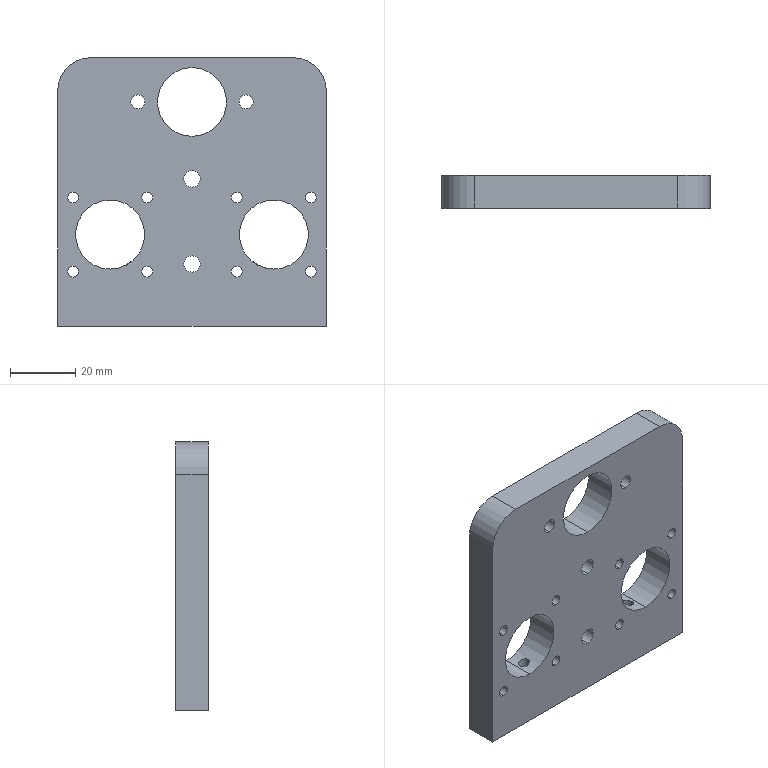Part | SolidWorks | features HoleWzd 7, Extrusion 1, Fillet 1, ICE 1, MirrorPattern 1 | 1 solid | 56 faces | box 82 x 10 x 82 mm | volume 53941 mm3 | cylinder 44 | plane 8 | cone 4 | commonest cylinder face diameters 3.3 x20 5 x8 4.3 x4 8 x4 21.1 x4 20 x2